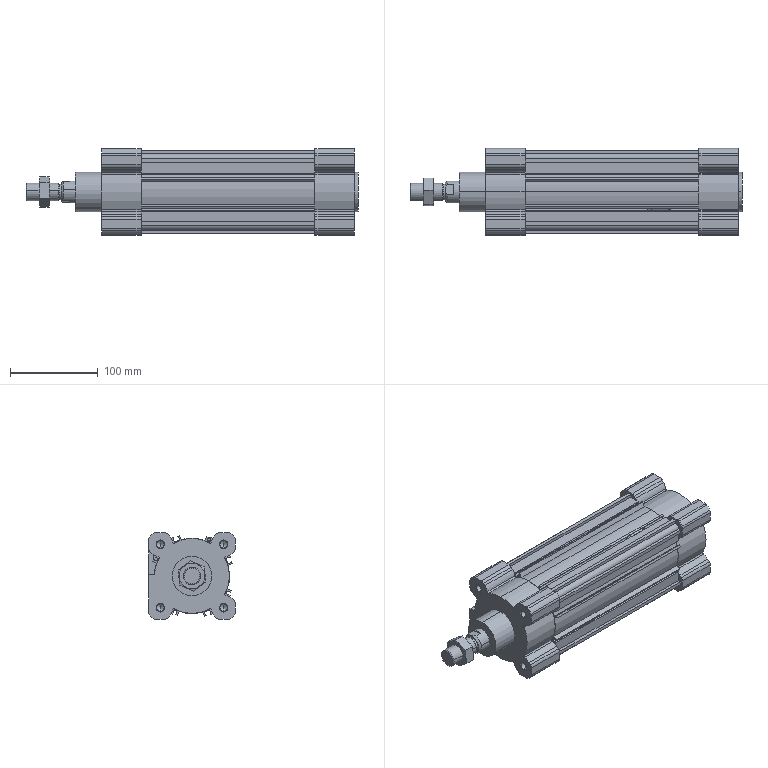Part | SolidWorks | 5 solids | 384 faces | box 378 x 99 x 99 mm | volume 1532576 mm3 | plane 175 | cylinder 154 | cone 55 | commonest cylinder face diameters 10 x30 3 x18 8.376 x16 28 x14 85.2 x10 4.25 x9